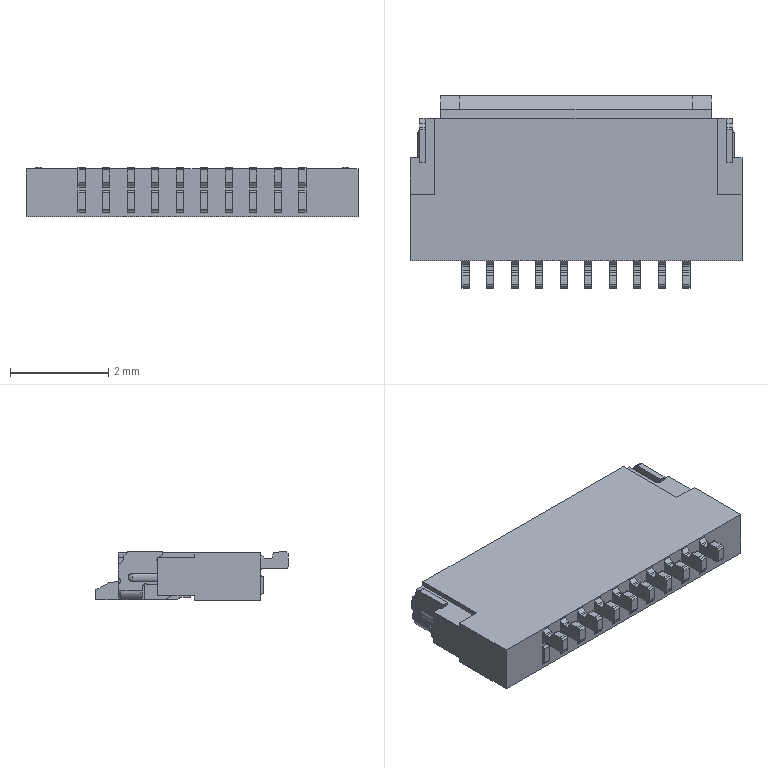Part | Creo | 1 solid | 539 faces | box 6.77 x 3.923 x 1 mm | volume 14.09 mm3 | plane 367 | cylinder 160 | sphere 4 | cone 4 | spline 2 | torus 2 | commonest cylinder face diameters 0.1 x120 0.2 x24 0.04 x4 0.28 x4 0.02 x2 0.125 x2